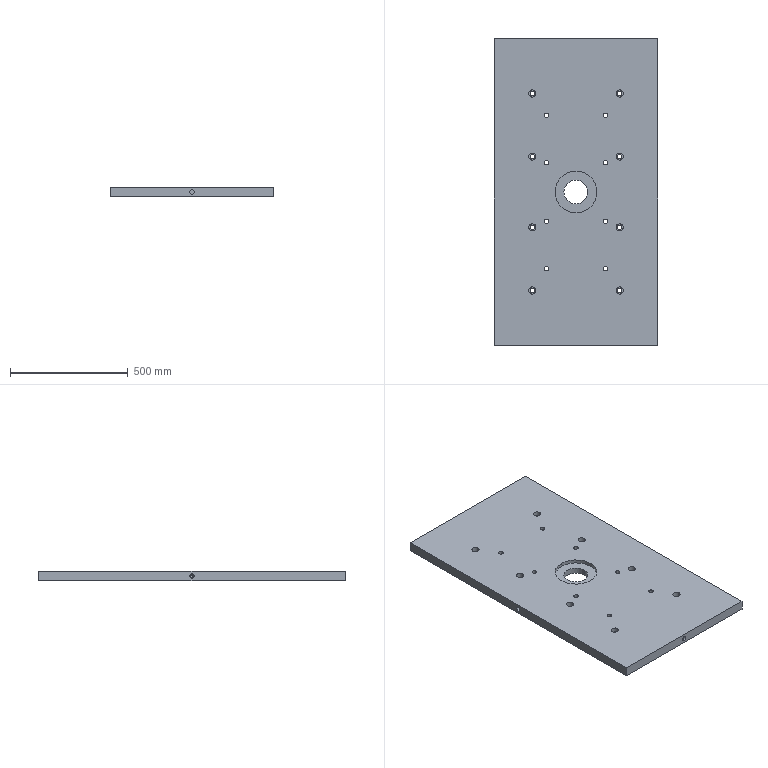Part | STEP file | 4-20.sldasm-Part-438 | 1 solid | 83 faces | box 692.15 x 1300 x 41.275 mm | volume 36245324 mm3 | cylinder 60 | plane 19 | cone 4 | commonest cylinder face diameters 19.05 x24 19.842 x16 30.162 x16 101.6 x2 177.8 x2